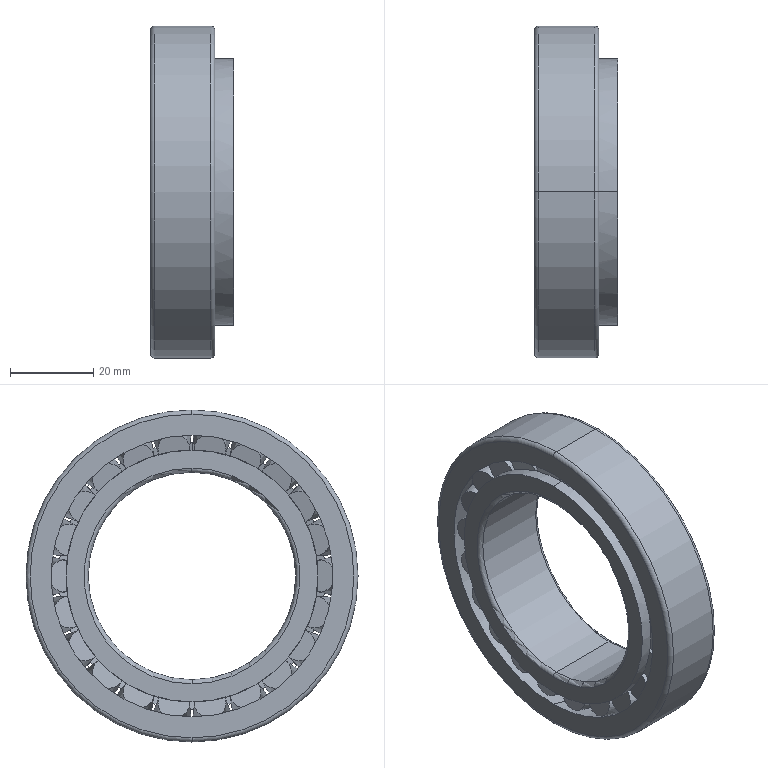Part | STEP file | Tapered Roller Bearing GB/T297-94 32010 | 1 solid | 179 faces | box 20 x 80 x 80 mm | volume 43880 mm3 | cone 115 | plane 48 | torus 8 | cylinder 8 | commonest cylinder face diameters 50 x2 60.705 x2 64.273 x2 80 x2